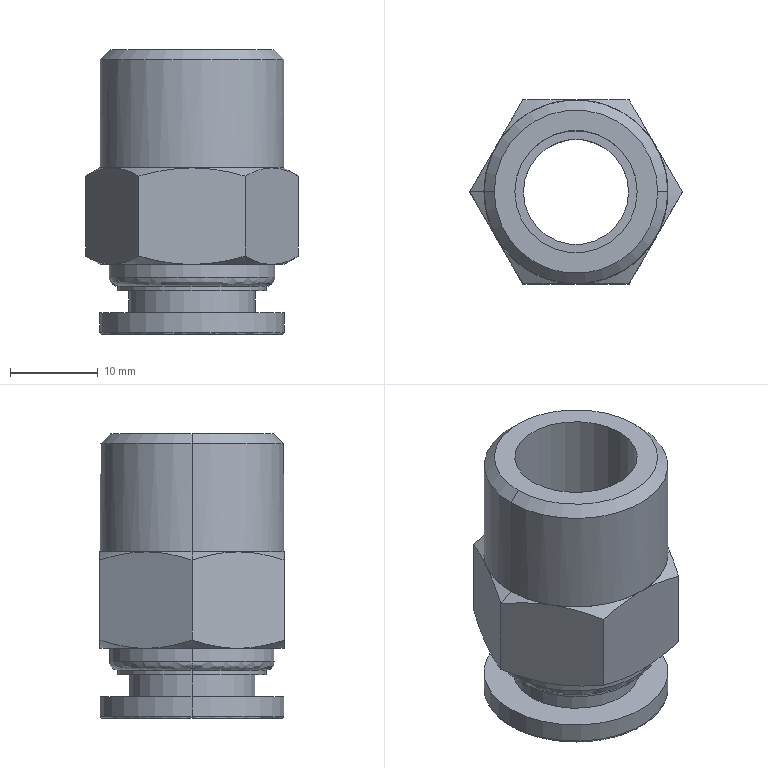Part | STEP file | APC12-04 | 1 solid | 47 faces | box 24.249 x 21 x 32.5 mm | volume 6609 mm3 | cone 16 | cylinder 14 | plane 13 | spline 4 | commonest cylinder face diameters 12 x2 13.97 x2 14.4 x2 16.9 x2 18.9 x2 20.955 x2